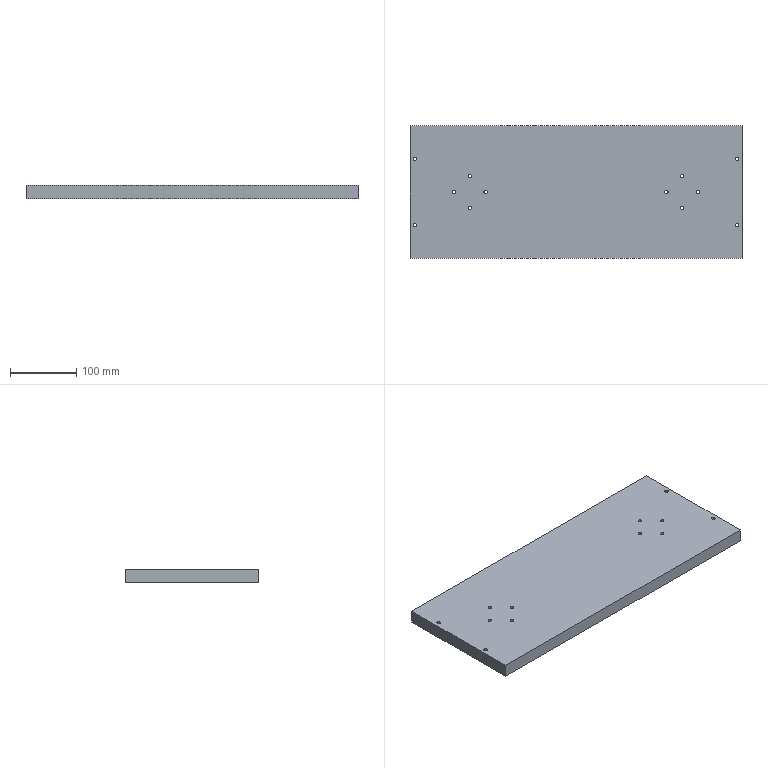Part | NX | features CBORE_HOLE 12, DATUM_CSYS 4, SKETCH 3, HOLE PACKAGE 2, EXTRUDE 1 | 1 solid | 42 faces | box 500 x 200 x 20 mm | volume 1988027 mm3 | cylinder 24 | plane 18 | commonest cylinder face diameters 5.2 x12 10 x12
STEP:
#1=CARTESIAN_POINT('',(-250.,100.,0.));
#2=VERTEX_POINT('',#1);
#3=CARTESIAN_POINT('',(-250.,-100.,0.));
#4=VERTEX_POINT('',#3);
#5=CARTESIAN_POINT('',(-250.,100.,0.));
#6=DIRECTION('',(0.,-1.,0.));
#7=VECTOR('',#6,1000.);
#8=LINE('',#5,#7);
#9=EDGE_CURVE('',#2,#4,#8,.T.);
#10=ORIENTED_EDGE('',*,*,#9,.T.);
#11=CARTESIAN_POINT('',(-250.,-100.,20.));
#12=VERTEX_POINT('',#11);
#13=CARTESIAN_POINT('',(-250.,-100.,20.));
#14=DIRECTION('',(0.,0.,-1.));
#15=VECTOR('',#14,1000.);
#16=LINE('',#13,#15);
#17=EDGE_CURVE('',#12,#4,#16,.T.);
#18=ORIENTED_EDGE('',*,*,#17,.F.);
#19=CARTESIAN_POINT('',(-250.,100.,20.));
#20=VERTEX_POINT('',#19);
#21=CARTESIAN_POINT('',(-250.,100.,20.));
#22=DIRECTION('',(0.,-1.,0.));
#23=VECTOR('',#22,1000.);
#24=LINE('',#21,#23);
#25=EDGE_CURVE('',#20,#12,#24,.T.);
#26=ORIENTED_EDGE('',*,*,#25,.F.);
#27=CARTESIAN_POINT('',(-250.,100.,20.));
#28=DIRECTION('',(0.,0.,-1.));
#29=VECTOR('',#28,1000.);
#30=LINE('',#27,#29);
#31=EDGE_CURVE('',#20,#2,#30,.T.);
#32=ORIENTED_EDGE('',*,*,#31,.T.);
#33=EDGE_LOOP('',(#10,#18,#26,#32));
#34=FACE_BOUND('',#33,.T.);
#35=CARTESIAN_POINT('',(-250.,100.,20.));
#36=DIRECTION('',(1.,0.,0.));
#37=DIRECTION('',(0.,1.,0.));
#38=AXIS2_PLACEMENT_3D('',#35,#36,#37);
#39=PLANE('',#38);
#40=ADVANCED_FACE('',(#34),#39,.F.);
#41=CARTESIAN_POINT('',(250.,-100.,0.));
#42=VERTEX_POINT('',#41);
#43=CARTESIAN_POINT('',(-250.,-100.,0.));
#44=DIRECTION('',(1.,0.,0.));
#45=VECTOR('',#44,1000.);
#46=LINE('',#43,#45);
#47=EDGE_CURVE('',#4,#42,#46,.T.);
#48=ORIENTED_EDGE('',*,*,#47,.T.);
#49=CARTESIAN_POINT('',(250.,-100.,20.));
#50=VERTEX_POINT('',#49);
#51=CARTESIAN_POINT('',(250.,-100.,20.));
#52=DIRECTION('',(0.,0.,-1.));
#53=VECTOR('',#52,1000.);
#54=LINE('',#51,#53);
#55=EDGE_CURVE('',#50,#42,#54,.T.);
#56=ORIENTED_EDGE('',*,*,#55,.F.);
#57=CARTESIAN_POINT('',(-250.,-100.,20.));
#58=DIRECTION('',(1.,0.,0.));
#59=VECTOR('',#58,1000.);
#60=LINE('',#57,#59);
#61=EDGE_CURVE('',#12,#50,#60,.T.);
#62=ORIENTED_EDGE('',*,*,#61,.F.);
#63=ORIENTED_EDGE('',*,*,#17,.T.);
#64=EDGE_LOOP('',(#48,#56,#62,#63));
#65=FACE_BOUND('',#64,.T.);
#66=CARTESIAN_POINT('',(-250.,-100.,20.));
#67=DIRECTION('',(0.,1.,0.));
#68=DIRECTION('',(0.,0.,1.));
#69=AXIS2_PLACEMENT_3D('',#66,#67,#68);
#70=PLANE('',#69);
#71=ADVANCED_FACE('',(#65),#70,.F.);
#72=CARTESIAN_POINT('',(250.,100.,0.));
#73=VERTEX_POINT('',#72);
#74=CARTESIAN_POINT('',(250.,-100.,0.));
#75=DIRECTION('',(0.,1.,0.));
#76=VECTOR('',#75,1000.);
#77=LINE('',#74,#76);
#78=EDGE_CURVE('',#42,#73,#77,.T.);
#79=ORIENTED_EDGE('',*,*,#78,.T.);
#80=CARTESIAN_POINT('',(250.,100.,20.));
#81=VERTEX_POINT('',#80);
#82=CARTESIAN_POINT('',(250.,100.,20.));
#83=DIRECTION('',(0.,0.,-1.));
#84=VECTOR('',#83,1000.);
#85=LINE('',#82,#84);
#86=EDGE_CURVE('',#81,#73,#85,.T.);
#87=ORIENTED_EDGE('',*,*,#86,.F.);
#88=CARTESIAN_POINT('',(250.,-100.,20.));
#89=DIRECTION('',(0.,1.,0.));
#90=VECTOR('',#89,1000.);
#91=LINE('',#88,#90);
#92=EDGE_CURVE('',#50,#81,#91,.T.);
#93=ORIENTED_EDGE('',*,*,#92,.F.);
#94=ORIENTED_EDGE('',*,*,#55,.T.);
#95=EDGE_LOOP('',(#79,#87,#93,#94));
#96=FACE_BOUND('',#95,.T.);
#97=CARTESIAN_POINT('',(250.,-100.,20.));
#98=DIRECTION('',(-1.,0.,0.));
#99=DIRECTION('',(0.,-1.,0.));
#100=AXIS2_PLACEMENT_3D('',#97,#98,#99);
#101=PLANE('',#100);
#102=ADVANCED_FACE('',(#96),#101,.F.);
#103=CARTESIAN_POINT('',(250.,100.,0.));
#104=DIRECTION('',(-1.,0.,0.));
#105=VECTOR('',#104,1000.);
#106=LINE('',#103,#105);
#107=EDGE_CURVE('',#73,#2,#106,.T.);
#108=ORIENTED_EDGE('',*,*,#107,.T.);
#109=ORIENTED_EDGE('',*,*,#31,.F.);
#110=CARTESIAN_POINT('',(250.,100.,20.));
#111=DIRECTION('',(-1.,0.,0.));
#112=VECTOR('',#111,1000.);
#113=LINE('',#110,#112);
#114=EDGE_CURVE('',#81,#20,#113,.T.);
#115=ORIENTED_EDGE('',*,*,#114,.F.);
#116=ORIENTED_EDGE('',*,*,#86,.T.);
#117=EDGE_LOOP('',(#108,#109,#115,#116));
#118=FACE_BOUND('',#117,.T.);
#119=CARTESIAN_POINT('',(250.,100.,20.));
#120=DIRECTION('',(0.,-1.,0.));
#121=DIRECTION('',(0.,0.,-1.));
#122=AXIS2_PLACEMENT_3D('',#119,#120,#121);
#123=PLANE('',#122);
#124=ADVANCED_FACE('',(#118),#123,.F.);
#125=CARTESIAN_POINT('',(-133.462,0.,20.));
#126=VERTEX_POINT('',#125);
#127=CARTESIAN_POINT('',(-136.062,0.,20.));
#128=DIRECTION('',(0.,0.,1.));
#129=DIRECTION('',(1.,0.,0.));
#130=AXIS2_PLACEMENT_3D('',#127,#128,#129);
#131=CIRCLE('',#130,2.6);
#132=EDGE_CURVE('',#126,#126,#131,.T.);
#133=ORIENTED_EDGE('',*,*,#132,.F.);
#134=EDGE_LOOP('',(#133));
#135=FACE_BOUND('',#134,.T.);
#136=CARTESIAN_POINT('',(-157.36,-23.75,20.));
#137=VERTEX_POINT('',#136);
#138=CARTESIAN_POINT('',(-159.96,-23.75,20.));
#139=DIRECTION('',(0.,0.,1.));
#140=DIRECTION('',(1.,0.,0.));
#141=AXIS2_PLACEMENT_3D('',#138,#139,#140);
#142=CIRCLE('',#141,2.6);
#143=EDGE_CURVE('',#137,#137,#142,.T.);
#144=ORIENTED_EDGE('',*,*,#143,.F.);
#145=EDGE_LOOP('',(#144));
#146=FACE_BOUND('',#145,.T.);
#147=CARTESIAN_POINT('',(-180.962,0.,20.));
#148=VERTEX_POINT('',#147);
#149=CARTESIAN_POINT('',(-183.562,0.,20.));
#150=DIRECTION('',(0.,0.,1.));
#151=DIRECTION('',(1.,0.,0.));
#152=AXIS2_PLACEMENT_3D('',#149,#150,#151);
#153=CIRCLE('',#152,2.6);
#154=EDGE_CURVE('',#148,#148,#153,.T.);
#155=ORIENTED_EDGE('',*,*,#154,.F.);
#156=EDGE_LOOP('',(#155));
#157=FACE_BOUND('',#156,.T.);
#158=CARTESIAN_POINT('',(-157.258,23.75,20.));
#159=VERTEX_POINT('',#158);
#160=CARTESIAN_POINT('',(-159.858,23.75,20.));
#161=DIRECTION('',(0.,0.,1.));
#162=DIRECTION('',(1.,0.,0.));
#163=AXIS2_PLACEMENT_3D('',#160,#161,#162);
#164=CIRCLE('',#163,2.6);
#165=EDGE_CURVE('',#159,#159,#164,.T.);
#166=ORIENTED_EDGE('',*,*,#165,.F.);
#167=EDGE_LOOP('',(#166));
#168=FACE_BOUND('',#167,.T.);
#169=CARTESIAN_POINT('',(138.662,0.,20.));
#170=VERTEX_POINT('',#169);
#171=CARTESIAN_POINT('',(136.062,0.,20.));
#172=DIRECTION('',(0.,0.,1.));
#173=DIRECTION('',(1.,0.,0.));
#174=AXIS2_PLACEMENT_3D('',#171,#172,#173);
#175=CIRCLE('',#174,2.6);
#176=EDGE_CURVE('',#170,#170,#175,.T.);
#177=ORIENTED_EDGE('',*,*,#176,.F.);
#178=EDGE_LOOP('',(#177));
#179=FACE_BOUND('',#178,.T.);
#180=CARTESIAN_POINT('',(162.56,-23.75,20.));
#181=VERTEX_POINT('',#180);
#182=CARTESIAN_POINT('',(159.96,-23.75,20.));
#183=DIRECTION('',(0.,0.,1.));
#184=DIRECTION('',(1.,0.,0.));
#185=AXIS2_PLACEMENT_3D('',#182,#183,#184);
#186=CIRCLE('',#185,2.6);
#187=EDGE_CURVE('',#181,#181,#186,.T.);
#188=ORIENTED_EDGE('',*,*,#187,.F.);
#189=EDGE_LOOP('',(#188));
#190=FACE_BOUND('',#189,.T.);
#191=CARTESIAN_POINT('',(186.162,0.,20.));
#192=VERTEX_POINT('',#191);
#193=CARTESIAN_POINT('',(183.562,0.,20.));
#194=DIRECTION('',(0.,0.,1.));
#195=DIRECTION('',(1.,0.,0.));
#196=AXIS2_PLACEMENT_3D('',#193,#194,#195);
#197=CIRCLE('',#196,2.6);
#198=EDGE_CURVE('',#192,#192,#197,.T.);
#199=ORIENTED_EDGE('',*,*,#198,.F.);
#200=EDGE_LOOP('',(#199));
#201=FACE_BOUND('',#200,.T.);
#202=CARTESIAN_POINT('',(162.458,23.75,20.));
#203=VERTEX_POINT('',#202);
#204=CARTESIAN_POINT('',(159.858,23.75,20.));
#205=DIRECTION('',(0.,0.,1.));
#206=DIRECTION('',(1.,0.,0.));
#207=AXIS2_PLACEMENT_3D('',#204,#205,#206);
#208=CIRCLE('',#207,2.6);
#209=EDGE_CURVE('',#203,#203,#208,.T.);
#210=ORIENTED_EDGE('',*,*,#209,.F.);
#211=EDGE_LOOP('',(#210));
#212=FACE_BOUND('',#211,.T.);
#213=CARTESIAN_POINT('',(-239.9,50.,20.));
#214=VERTEX_POINT('',#213);
#215=CARTESIAN_POINT('',(-242.5,50.,20.));
#216=DIRECTION('',(0.,0.,1.));
#217=DIRECTION('',(1.,0.,0.));
#218=AXIS2_PLACEMENT_3D('',#215,#216,#217);
#219=CIRCLE('',#218,2.6);
#220=EDGE_CURVE('',#214,#214,#219,.T.);
#221=ORIENTED_EDGE('',*,*,#220,.F.);
#222=EDGE_LOOP('',(#221));
#223=FACE_BOUND('',#222,.T.);
#224=CARTESIAN_POINT('',(-239.9,-50.,20.));
#225=VERTEX_POINT('',#224);
#226=CARTESIAN_POINT('',(-242.5,-50.,20.));
#227=DIRECTION('',(0.,0.,1.));
#228=DIRECTION('',(1.,0.,0.));
#229=AXIS2_PLACEMENT_3D('',#226,#227,#228);
#230=CIRCLE('',#229,2.6);
#231=EDGE_CURVE('',#225,#225,#230,.T.);
#232=ORIENTED_EDGE('',*,*,#231,.F.);
#233=EDGE_LOOP('',(#232));
#234=FACE_BOUND('',#233,.T.);
#235=CARTESIAN_POINT('',(245.1,50.,20.));
#236=VERTEX_POINT('',#235);
#237=CARTESIAN_POINT('',(242.5,50.,20.));
#238=DIRECTION('',(0.,0.,1.));
#239=DIRECTION('',(1.,0.,0.));
#240=AXIS2_PLACEMENT_3D('',#237,#238,#239);
#241=CIRCLE('',#240,2.6);
#242=EDGE_CURVE('',#236,#236,#241,.T.);
#243=ORIENTED_EDGE('',*,*,#242,.F.);
#244=EDGE_LOOP('',(#243));
#245=FACE_BOUND('',#244,.T.);
#246=CARTESIAN_POINT('',(245.1,-50.,20.));
#247=VERTEX_POINT('',#246);
#248=CARTESIAN_POINT('',(242.5,-50.,20.));
#249=DIRECTION('',(0.,0.,1.));
#250=DIRECTION('',(1.,0.,0.));
#251=AXIS2_PLACEMENT_3D('',#248,#249,#250);
#252=CIRCLE('',#251,2.6);
#253=EDGE_CURVE('',#247,#247,#252,.T.);
#254=ORIENTED_EDGE('',*,*,#253,.F.);
#255=EDGE_LOOP('',(#254));
#256=FACE_BOUND('',#255,.T.);
#257=ORIENTED_EDGE('',*,*,#25,.T.);
#258=ORIENTED_EDGE('',*,*,#61,.T.);
#259=ORIENTED_EDGE('',*,*,#92,.T.);
#260=ORIENTED_EDGE('',*,*,#114,.T.);
#261=EDGE_LOOP('',(#257,#258,#259,#260));
#262=FACE_BOUND('',#261,.T.);
#263=CARTESIAN_POINT('',(0.,0.,20.));
#264=DIRECTION('',(0.,0.,1.));
#265=DIRECTION('',(1.,0.,0.));
#266=AXIS2_PLACEMENT_3D('',#263,#264,#265);
#267=PLANE('',#266);
#268=ADVANCED_FACE('',(#135,#146,#157,#168,#179,#190,#201,#212,#223,#234,#245,#256,#262),#267,.T.);
#269=CARTESIAN_POINT('',(-131.062,0.,0.));
#270=VERTEX_POINT('',#269);
#271=CARTESIAN_POINT('',(-136.062,0.,0.));
#272=DIRECTION('',(0.,0.,1.));
#273=DIRECTION('',(1.,0.,0.));
#274=AXIS2_PLACEMENT_3D('',#271,#272,#273);
#275=CIRCLE('',#274,5.);
#276=EDGE_CURVE('',#270,#270,#275,.T.);
#277=ORIENTED_EDGE('',*,*,#276,.T.);
#278=EDGE_LOOP('',(#277));
#279=FACE_BOUND('',#278,.T.);
#280=CARTESIAN_POINT('',(-154.96,-23.75,0.));
#281=VERTEX_POINT('',#280);
#282=CARTESIAN_POINT('',(-159.96,-23.75,0.));
#283=DIRECTION('',(0.,0.,1.));
#284=DIRECTION('',(1.,0.,0.));
#285=AXIS2_PLACEMENT_3D('',#282,#283,#284);
#286=CIRCLE('',#285,5.);
#287=EDGE_CURVE('',#281,#281,#286,.T.);
#288=ORIENTED_EDGE('',*,*,#287,.T.);
#289=EDGE_LOOP('',(#288));
#290=FACE_BOUND('',#289,.T.);
#291=CARTESIAN_POINT('',(-178.562,0.,0.));
#292=VERTEX_POINT('',#291);
#293=CARTESIAN_POINT('',(-183.562,0.,0.));
#294=DIRECTION('',(0.,0.,1.));
#295=DIRECTION('',(1.,0.,0.));
#296=AXIS2_PLACEMENT_3D('',#293,#294,#295);
#297=CIRCLE('',#296,5.);
#298=EDGE_CURVE('',#292,#292,#297,.T.);
#299=ORIENTED_EDGE('',*,*,#298,.T.);
#300=EDGE_LOOP('',(#299));
#301=FACE_BOUND('',#300,.T.);
#302=CARTESIAN_POINT('',(-154.858,23.75,0.));
#303=VERTEX_POINT('',#302);
#304=CARTESIAN_POINT('',(-159.858,23.75,0.));
#305=DIRECTION('',(0.,0.,1.));
#306=DIRECTION('',(1.,0.,0.));
#307=AXIS2_PLACEMENT_3D('',#304,#305,#306);
#308=CIRCLE('',#307,5.);
#309=EDGE_CURVE('',#303,#303,#308,.T.);
#310=ORIENTED_EDGE('',*,*,#309,.T.);
#311=EDGE_LOOP('',(#310));
#312=FACE_BOUND('',#311,.T.);
#313=CARTESIAN_POINT('',(141.062,0.,0.));
#314=VERTEX_POINT('',#313);
#315=CARTESIAN_POINT('',(136.062,0.,0.));
#316=DIRECTION('',(0.,0.,1.));
#317=DIRECTION('',(1.,0.,0.));
#318=AXIS2_PLACEMENT_3D('',#315,#316,#317);
#319=CIRCLE('',#318,5.);
#320=EDGE_CURVE('',#314,#314,#319,.T.);
#321=ORIENTED_EDGE('',*,*,#320,.T.);
#322=EDGE_LOOP('',(#321));
#323=FACE_BOUND('',#322,.T.);
#324=CARTESIAN_POINT('',(164.96,-23.75,0.));
#325=VERTEX_POINT('',#324);
#326=CARTESIAN_POINT('',(159.96,-23.75,0.));
#327=DIRECTION('',(0.,0.,1.));
#328=DIRECTION('',(1.,0.,0.));
#329=AXIS2_PLACEMENT_3D('',#326,#327,#328);
#330=CIRCLE('',#329,5.);
#331=EDGE_CURVE('',#325,#325,#330,.T.);
#332=ORIENTED_EDGE('',*,*,#331,.T.);
#333=EDGE_LOOP('',(#332));
#334=FACE_BOUND('',#333,.T.);
#335=CARTESIAN_POINT('',(188.562,0.,0.));
#336=VERTEX_POINT('',#335);
#337=CARTESIAN_POINT('',(183.562,0.,0.));
#338=DIRECTION('',(0.,0.,1.));
#339=DIRECTION('',(1.,0.,0.));
#340=AXIS2_PLACEMENT_3D('',#337,#338,#339);
#341=CIRCLE('',#340,5.);
#342=EDGE_CURVE('',#336,#336,#341,.T.);
#343=ORIENTED_EDGE('',*,*,#342,.T.);
#344=EDGE_LOOP('',(#343));
#345=FACE_BOUND('',#344,.T.);
#346=CARTESIAN_POINT('',(164.858,23.75,0.));
#347=VERTEX_POINT('',#346);
#348=CARTESIAN_POINT('',(159.858,23.75,0.));
#349=DIRECTION('',(0.,0.,1.));
#350=DIRECTION('',(1.,0.,0.));
#351=AXIS2_PLACEMENT_3D('',#348,#349,#350);
#352=CIRCLE('',#351,5.);
#353=EDGE_CURVE('',#347,#347,#352,.T.);
#354=ORIENTED_EDGE('',*,*,#353,.T.);
#355=EDGE_LOOP('',(#354));
#356=FACE_BOUND('',#355,.T.);
#357=CARTESIAN_POINT('',(-237.5,50.,0.));
#358=VERTEX_POINT('',#357);
#359=CARTESIAN_POINT('',(-242.5,50.,0.));
#360=DIRECTION('',(0.,0.,1.));
#361=DIRECTION('',(1.,0.,0.));
#362=AXIS2_PLACEMENT_3D('',#359,#360,#361);
#363=CIRCLE('',#362,5.);
#364=EDGE_CURVE('',#358,#358,#363,.T.);
#365=ORIENTED_EDGE('',*,*,#364,.T.);
#366=EDGE_LOOP('',(#365));
#367=FACE_BOUND('',#366,.T.);
#368=CARTESIAN_POINT('',(-237.5,-50.,0.));
#369=VERTEX_POINT('',#368);
#370=CARTESIAN_POINT('',(-242.5,-50.,0.));
#371=DIRECTION('',(0.,0.,1.));
#372=DIRECTION('',(1.,0.,0.));
#373=AXIS2_PLACEMENT_3D('',#370,#371,#372);
#374=CIRCLE('',#373,5.);
#375=EDGE_CURVE('',#369,#369,#374,.T.);
#376=ORIENTED_EDGE('',*,*,#375,.T.);
#377=EDGE_LOOP('',(#376));
#378=FACE_BOUND('',#377,.T.);
#379=CARTESIAN_POINT('',(247.5,50.,0.));
#380=VERTEX_POINT('',#379);
#381=CARTESIAN_POINT('',(242.5,50.,0.));
#382=DIRECTION('',(0.,0.,1.));
#383=DIRECTION('',(1.,0.,0.));
#384=AXIS2_PLACEMENT_3D('',#381,#382,#383);
#385=CIRCLE('',#384,5.);
#386=EDGE_CURVE('',#380,#380,#385,.T.);
#387=ORIENTED_EDGE('',*,*,#386,.T.);
#388=EDGE_LOOP('',(#387));
#389=FACE_BOUND('',#388,.T.);
#390=CARTESIAN_POINT('',(247.5,-50.,0.));
#391=VERTEX_POINT('',#390);
#392=CARTESIAN_POINT('',(242.5,-50.,0.));
#393=DIRECTION('',(0.,0.,1.));
#394=DIRECTION('',(1.,0.,0.));
#395=AXIS2_PLACEMENT_3D('',#392,#393,#394);
#396=CIRCLE('',#395,5.);
#397=EDGE_CURVE('',#391,#391,#396,.T.);
#398=ORIENTED_EDGE('',*,*,#397,.T.);
#399=EDGE_LOOP('',(#398));
#400=FACE_BOUND('',#399,.T.);
#401=ORIENTED_EDGE('',*,*,#9,.F.);
#402=ORIENTED_EDGE('',*,*,#107,.F.);
#403=ORIENTED_EDGE('',*,*,#78,.F.);
#404=ORIENTED_EDGE('',*,*,#47,.F.);
#405=EDGE_LOOP('',(#401,#402,#403,#404));
#406=FACE_BOUND('',#405,.T.);
#407=CARTESIAN_POINT('',(0.,0.,0.));
#408=DIRECTION('',(0.,0.,1.));
#409=DIRECTION('',(1.,0.,0.));
#410=AXIS2_PLACEMENT_3D('',#407,#408,#409);
#411=PLANE('',#410);
#412=ADVANCED_FACE('',(#279,#290,#301,#312,#323,#334,#345,#356,#367,#378,#389,#400,#406),#411,.F.);
#413=ORIENTED_EDGE('',*,*,#253,.T.);
#414=EDGE_LOOP('',(#413));
#415=FACE_BOUND('',#414,.T.);
#416=CARTESIAN_POINT('',(245.1,-50.,10.));
#417=VERTEX_POINT('',#416);
#418=CARTESIAN_POINT('',(242.5,-50.,10.));
#419=DIRECTION('',(0.,0.,1.));
#420=DIRECTION('',(1.,0.,0.));
#421=AXIS2_PLACEMENT_3D('',#418,#419,#420);
#422=CIRCLE('',#421,2.6);
#423=EDGE_CURVE('',#417,#417,#422,.F.);
#424=ORIENTED_EDGE('',*,*,#423,.T.);
#425=EDGE_LOOP('',(#424));
#426=FACE_BOUND('',#425,.T.);
#427=CARTESIAN_POINT('',(242.5,-50.,50.));
#428=DIRECTION('',(0.,0.,1.));
#429=DIRECTION('',(1.,0.,0.));
#430=AXIS2_PLACEMENT_3D('',#427,#428,#429);
#431=CYLINDRICAL_SURFACE('',#430,2.6);
#432=ADVANCED_FACE('',(#415,#426),#431,.F.);
#433=ORIENTED_EDGE('',*,*,#423,.F.);
#434=EDGE_LOOP('',(#433));
#435=FACE_BOUND('',#434,.T.);
#436=CARTESIAN_POINT('',(247.5,-50.,10.));
#437=VERTEX_POINT('',#436);
#438=CARTESIAN_POINT('',(242.5,-50.,10.));
#439=DIRECTION('',(0.,0.,1.));
#440=DIRECTION('',(1.,0.,0.));
#441=AXIS2_PLACEMENT_3D('',#438,#439,#440);
#442=CIRCLE('',#441,5.);
#443=EDGE_CURVE('',#437,#437,#442,.F.);
#444=ORIENTED_EDGE('',*,*,#443,.T.);
#445=EDGE_LOOP('',(#444));
#446=FACE_BOUND('',#445,.T.);
#447=CARTESIAN_POINT('',(242.5,-50.,10.));
#448=DIRECTION('',(0.,0.,1.));
#449=DIRECTION('',(1.,0.,0.));
#450=AXIS2_PLACEMENT_3D('',#447,#448,#449);
#451=PLANE('',#450);
#452=ADVANCED_FACE('',(#435,#446),#451,.F.);
#453=ORIENTED_EDGE('',*,*,#443,.F.);
#454=EDGE_LOOP('',(#453));
#455=FACE_BOUND('',#454,.T.);
#456=ORIENTED_EDGE('',*,*,#397,.F.);
#457=EDGE_LOOP('',(#456));
#458=FACE_BOUND('',#457,.T.);
#459=CARTESIAN_POINT('',(242.5,-50.,0.));
#460=DIRECTION('',(0.,0.,1.));
#461=DIRECTION('',(1.,0.,0.));
#462=AXIS2_PLACEMENT_3D('',#459,#460,#461);
#463=CYLINDRICAL_SURFACE('',#462,5.);
#464=ADVANCED_FACE('',(#455,#458),#463,.F.);
#465=ORIENTED_EDGE('',*,*,#242,.T.);
#466=EDGE_LOOP('',(#465));
#467=FACE_BOUND('',#466,.T.);
#468=CARTESIAN_POINT('',(245.1,50.,10.));
#469=VERTEX_POINT('',#468);
#470=CARTESIAN_POINT('',(242.5,50.,10.));
#471=DIRECTION('',(0.,0.,1.));
#472=DIRECTION('',(1.,0.,0.));
#473=AXIS2_PLACEMENT_3D('',#470,#471,#472);
#474=CIRCLE('',#473,2.6);
#475=EDGE_CURVE('',#469,#469,#474,.F.);
#476=ORIENTED_EDGE('',*,*,#475,.T.);
#477=EDGE_LOOP('',(#476));
#478=FACE_BOUND('',#477,.T.);
#479=CARTESIAN_POINT('',(242.5,50.,50.));
#480=DIRECTION('',(0.,0.,1.));
#481=DIRECTION('',(1.,0.,0.));
#482=AXIS2_PLACEMENT_3D('',#479,#480,#481);
#483=CYLINDRICAL_SURFACE('',#482,2.6);
#484=ADVANCED_FACE('',(#467,#478),#483,.F.);
#485=ORIENTED_EDGE('',*,*,#475,.F.);
#486=EDGE_LOOP('',(#485));
#487=FACE_BOUND('',#486,.T.);
#488=CARTESIAN_POINT('',(247.5,50.,10.));
#489=VERTEX_POINT('',#488);
#490=CARTESIAN_POINT('',(242.5,50.,10.));
#491=DIRECTION('',(0.,0.,1.));
#492=DIRECTION('',(1.,0.,0.));
#493=AXIS2_PLACEMENT_3D('',#490,#491,#492);
#494=CIRCLE('',#493,5.);
#495=EDGE_CURVE('',#489,#489,#494,.F.);
#496=ORIENTED_EDGE('',*,*,#495,.T.);
#497=EDGE_LOOP('',(#496));
#498=FACE_BOUND('',#497,.T.);
#499=CARTESIAN_POINT('',(242.5,50.,10.));
#500=DIRECTION('',(0.,0.,1.));
#501=DIRECTION('',(1.,0.,0.));
#502=AXIS2_PLACEMENT_3D('',#499,#500,#501);
#503=PLANE('',#502);
#504=ADVANCED_FACE('',(#487,#498),#503,.F.);
#505=ORIENTED_EDGE('',*,*,#495,.F.);
#506=EDGE_LOOP('',(#505));
#507=FACE_BOUND('',#506,.T.);
#508=ORIENTED_EDGE('',*,*,#386,.F.);
#509=EDGE_LOOP('',(#508));
#510=FACE_BOUND('',#509,.T.);
#511=CARTESIAN_POINT('',(242.5,50.,0.));
#512=DIRECTION('',(0.,0.,1.));
#513=DIRECTION('',(1.,0.,0.));
#514=AXIS2_PLACEMENT_3D('',#511,#512,#513);
#515=CYLINDRICAL_SURFACE('',#514,5.);
#516=ADVANCED_FACE('',(#507,#510),#515,.F.);
#517=ORIENTED_EDGE('',*,*,#231,.T.);
#518=EDGE_LOOP('',(#517));
#519=FACE_BOUND('',#518,.T.);
#520=CARTESIAN_POINT('',(-239.9,-50.,10.));
#521=VERTEX_POINT('',#520);
#522=CARTESIAN_POINT('',(-242.5,-50.,10.));
#523=DIRECTION('',(0.,0.,1.));
#524=DIRECTION('',(1.,0.,0.));
#525=AXIS2_PLACEMENT_3D('',#522,#523,#524);
#526=CIRCLE('',#525,2.6);
#527=EDGE_CURVE('',#521,#521,#526,.F.);
#528=ORIENTED_EDGE('',*,*,#527,.T.);
#529=EDGE_LOOP('',(#528));
#530=FACE_BOUND('',#529,.T.);
#531=CARTESIAN_POINT('',(-242.5,-50.,50.));
#532=DIRECTION('',(0.,0.,1.));
#533=DIRECTION('',(1.,0.,0.));
#534=AXIS2_PLACEMENT_3D('',#531,#532,#533);
#535=CYLINDRICAL_SURFACE('',#534,2.6);
#536=ADVANCED_FACE('',(#519,#530),#535,.F.);
#537=ORIENTED_EDGE('',*,*,#527,.F.);
#538=EDGE_LOOP('',(#537));
#539=FACE_BOUND('',#538,.T.);
#540=CARTESIAN_POINT('',(-237.5,-50.,10.));
#541=VERTEX_POINT('',#540);
#542=CARTESIAN_POINT('',(-242.5,-50.,10.));
#543=DIRECTION('',(0.,0.,1.));
#544=DIRECTION('',(1.,0.,0.));
#545=AXIS2_PLACEMENT_3D('',#542,#543,#544);
#546=CIRCLE('',#545,5.);
#547=EDGE_CURVE('',#541,#541,#546,.F.);
#548=ORIENTED_EDGE('',*,*,#547,.T.);
#549=EDGE_LOOP('',(#548));
#550=FACE_BOUND('',#549,.T.);
#551=CARTESIAN_POINT('',(-242.5,-50.,10.));
#552=DIRECTION('',(0.,0.,1.));
#553=DIRECTION('',(1.,0.,0.));
#554=AXIS2_PLACEMENT_3D('',#551,#552,#553);
#555=PLANE('',#554);
#556=ADVANCED_FACE('',(#539,#550),#555,.F.);
#557=ORIENTED_EDGE('',*,*,#547,.F.);
#558=EDGE_LOOP('',(#557));
#559=FACE_BOUND('',#558,.T.);
#560=ORIENTED_EDGE('',*,*,#375,.F.);
#561=EDGE_LOOP('',(#560));
#562=FACE_BOUND('',#561,.T.);
#563=CARTESIAN_POINT('',(-242.5,-50.,0.));
#564=DIRECTION('',(0.,0.,1.));
#565=DIRECTION('',(1.,0.,0.));
#566=AXIS2_PLACEMENT_3D('',#563,#564,#565);
#567=CYLINDRICAL_SURFACE('',#566,5.);
#568=ADVANCED_FACE('',(#559,#562),#567,.F.);
#569=ORIENTED_EDGE('',*,*,#220,.T.);
#570=EDGE_LOOP('',(#569));
#571=FACE_BOUND('',#570,.T.);
#572=CARTESIAN_POINT('',(-239.9,50.,10.));
#573=VERTEX_POINT('',#572);
#574=CARTESIAN_POINT('',(-242.5,50.,10.));
#575=DIRECTION('',(0.,0.,1.));
#576=DIRECTION('',(1.,0.,0.));
#577=AXIS2_PLACEMENT_3D('',#574,#575,#576);
#578=CIRCLE('',#577,2.6);
#579=EDGE_CURVE('',#573,#573,#578,.F.);
#580=ORIENTED_EDGE('',*,*,#579,.T.);
#581=EDGE_LOOP('',(#580));
#582=FACE_BOUND('',#581,.T.);
#583=CARTESIAN_POINT('',(-242.5,50.,50.));
#584=DIRECTION('',(0.,0.,1.));
#585=DIRECTION('',(1.,0.,0.));
#586=AXIS2_PLACEMENT_3D('',#583,#584,#585);
#587=CYLINDRICAL_SURFACE('',#586,2.6);
#588=ADVANCED_FACE('',(#571,#582),#587,.F.);
#589=ORIENTED_EDGE('',*,*,#579,.F.);
#590=EDGE_LOOP('',(#589));
#591=FACE_BOUND('',#590,.T.);
#592=CARTESIAN_POINT('',(-237.5,50.,10.));
#593=VERTEX_POINT('',#592);
#594=CARTESIAN_POINT('',(-242.5,50.,10.));
#595=DIRECTION('',(0.,0.,1.));
#596=DIRECTION('',(1.,0.,0.));
#597=AXIS2_PLACEMENT_3D('',#594,#595,#596);
#598=CIRCLE('',#597,5.);
#599=EDGE_CURVE('',#593,#593,#598,.F.);
#600=ORIENTED_EDGE('',*,*,#599,.T.);
#601=EDGE_LOOP('',(#600));
#602=FACE_BOUND('',#601,.T.);
#603=CARTESIAN_POINT('',(-242.5,50.,10.));
#604=DIRECTION('',(0.,0.,1.));
#605=DIRECTION('',(1.,0.,0.));
#606=AXIS2_PLACEMENT_3D('',#603,#604,#605);
#607=PLANE('',#606);
#608=ADVANCED_FACE('',(#591,#602),#607,.F.);
#609=ORIENTED_EDGE('',*,*,#599,.F.);
#610=EDGE_LOOP('',(#609));
#611=FACE_BOUND('',#610,.T.);
#612=ORIENTED_EDGE('',*,*,#364,.F.);
#613=EDGE_LOOP('',(#612));
#614=FACE_BOUND('',#613,.T.);
#615=CARTESIAN_POINT('',(-242.5,50.,0.));
#616=DIRECTION('',(0.,0.,1.));
#617=DIRECTION('',(1.,0.,0.));
#618=AXIS2_PLACEMENT_3D('',#615,#616,#617);
#619=CYLINDRICAL_SURFACE('',#618,5.);
#620=ADVANCED_FACE('',(#611,#614),#619,.F.);
#621=ORIENTED_EDGE('',*,*,#209,.T.);
#622=EDGE_LOOP('',(#621));
#623=FACE_BOUND('',#622,.T.);
#624=CARTESIAN_POINT('',(162.458,23.75,10.));
#625=VERTEX_POINT('',#624);
#626=CARTESIAN_POINT('',(159.858,23.75,10.));
#627=DIRECTION('',(0.,0.,1.));
#628=DIRECTION('',(1.,0.,0.));
#629=AXIS2_PLACEMENT_3D('',#626,#627,#628);
#630=CIRCLE('',#629,2.6);
#631=EDGE_CURVE('',#625,#625,#630,.F.);
#632=ORIENTED_EDGE('',*,*,#631,.T.);
#633=EDGE_LOOP('',(#632));
#634=FACE_BOUND('',#633,.T.);
#635=CARTESIAN_POINT('',(159.858,23.75,50.));
#636=DIRECTION('',(0.,0.,1.));
#637=DIRECTION('',(1.,0.,0.));
#638=AXIS2_PLACEMENT_3D('',#635,#636,#637);
#639=CYLINDRICAL_SURFACE('',#638,2.6);
#640=ADVANCED_FACE('',(#623,#634),#639,.F.);
#641=ORIENTED_EDGE('',*,*,#631,.F.);
#642=EDGE_LOOP('',(#641));
#643=FACE_BOUND('',#642,.T.);
#644=CARTESIAN_POINT('',(164.858,23.75,10.));
#645=VERTEX_POINT('',#644);
#646=CARTESIAN_POINT('',(159.858,23.75,10.));
#647=DIRECTION('',(0.,0.,1.));
#648=DIRECTION('',(1.,0.,0.));
#649=AXIS2_PLACEMENT_3D('',#646,#647,#648);
#650=CIRCLE('',#649,5.);
#651=EDGE_CURVE('',#645,#645,#650,.F.);
#652=ORIENTED_EDGE('',*,*,#651,.T.);
#653=EDGE_LOOP('',(#652));
#654=FACE_BOUND('',#653,.T.);
#655=CARTESIAN_POINT('',(159.858,23.75,10.));
#656=DIRECTION('',(0.,0.,1.));
#657=DIRECTION('',(1.,0.,0.));
#658=AXIS2_PLACEMENT_3D('',#655,#656,#657);
#659=PLANE('',#658);
#660=ADVANCED_FACE('',(#643,#654),#659,.F.);
#661=ORIENTED_EDGE('',*,*,#651,.F.);
#662=EDGE_LOOP('',(#661));
#663=FACE_BOUND('',#662,.T.);
#664=ORIENTED_EDGE('',*,*,#353,.F.);
#665=EDGE_LOOP('',(#664));
#666=FACE_BOUND('',#665,.T.);
#667=CARTESIAN_POINT('',(159.858,23.75,0.));
#668=DIRECTION('',(0.,0.,1.));
#669=DIRECTION('',(1.,0.,0.));
#670=AXIS2_PLACEMENT_3D('',#667,#668,#669);
#671=CYLINDRICAL_SURFACE('',#670,5.);
#672=ADVANCED_FACE('',(#663,#666),#671,.F.);
#673=ORIENTED_EDGE('',*,*,#198,.T.);
#674=EDGE_LOOP('',(#673));
#675=FACE_BOUND('',#674,.T.);
#676=CARTESIAN_POINT('',(186.162,0.,10.));
#677=VERTEX_POINT('',#676);
#678=CARTESIAN_POINT('',(183.562,0.,10.));
#679=DIRECTION('',(0.,0.,1.));
#680=DIRECTION('',(1.,0.,0.));
#681=AXIS2_PLACEMENT_3D('',#678,#679,#680);
#682=CIRCLE('',#681,2.6);
#683=EDGE_CURVE('',#677,#677,#682,.F.);
#684=ORIENTED_EDGE('',*,*,#683,.T.);
#685=EDGE_LOOP('',(#684));
#686=FACE_BOUND('',#685,.T.);
#687=CARTESIAN_POINT('',(183.562,0.,50.));
#688=DIRECTION('',(0.,0.,1.));
#689=DIRECTION('',(1.,0.,0.));
#690=AXIS2_PLACEMENT_3D('',#687,#688,#689);
#691=CYLINDRICAL_SURFACE('',#690,2.6);
#692=ADVANCED_FACE('',(#675,#686),#691,.F.);
#693=ORIENTED_EDGE('',*,*,#683,.F.);
#694=EDGE_LOOP('',(#693));
#695=FACE_BOUND('',#694,.T.);
#696=CARTESIAN_POINT('',(188.562,0.,10.));
#697=VERTEX_POINT('',#696);
#698=CARTESIAN_POINT('',(183.562,0.,10.));
#699=DIRECTION('',(0.,0.,1.));
#700=DIRECTION('',(1.,0.,0.));
#701=AXIS2_PLACEMENT_3D('',#698,#699,#700);
#702=CIRCLE('',#701,5.);
#703=EDGE_CURVE('',#697,#697,#702,.F.);
#704=ORIENTED_EDGE('',*,*,#703,.T.);
#705=EDGE_LOOP('',(#704));
#706=FACE_BOUND('',#705,.T.);
#707=CARTESIAN_POINT('',(183.562,0.,10.));
#708=DIRECTION('',(0.,0.,1.));
#709=DIRECTION('',(1.,0.,0.));
#710=AXIS2_PLACEMENT_3D('',#707,#708,#709);
#711=PLANE('',#710);
#712=ADVANCED_FACE('',(#695,#706),#711,.F.);
#713=ORIENTED_EDGE('',*,*,#703,.F.);
#714=EDGE_LOOP('',(#713));
#715=FACE_BOUND('',#714,.T.);
#716=ORIENTED_EDGE('',*,*,#342,.F.);
#717=EDGE_LOOP('',(#716));
#718=FACE_BOUND('',#717,.T.);
#719=CARTESIAN_POINT('',(183.562,0.,0.));
#720=DIRECTION('',(0.,0.,1.));
#721=DIRECTION('',(1.,0.,0.));
#722=AXIS2_PLACEMENT_3D('',#719,#720,#721);
#723=CYLINDRICAL_SURFACE('',#722,5.);
#724=ADVANCED_FACE('',(#715,#718),#723,.F.);
#725=ORIENTED_EDGE('',*,*,#187,.T.);
#726=EDGE_LOOP('',(#725));
#727=FACE_BOUND('',#726,.T.);
#728=CARTESIAN_POINT('',(162.56,-23.75,10.));
#729=VERTEX_POINT('',#728);
#730=CARTESIAN_POINT('',(159.96,-23.75,10.));
#731=DIRECTION('',(0.,0.,1.));
#732=DIRECTION('',(1.,0.,0.));
#733=AXIS2_PLACEMENT_3D('',#730,#731,#732);
#734=CIRCLE('',#733,2.6);
#735=EDGE_CURVE('',#729,#729,#734,.F.);
#736=ORIENTED_EDGE('',*,*,#735,.T.);
#737=EDGE_LOOP('',(#736));
#738=FACE_BOUND('',#737,.T.);
#739=CARTESIAN_POINT('',(159.96,-23.75,50.));
#740=DIRECTION('',(0.,0.,1.));
#741=DIRECTION('',(1.,0.,0.));
#742=AXIS2_PLACEMENT_3D('',#739,#740,#741);
#743=CYLINDRICAL_SURFACE('',#742,2.6);
#744=ADVANCED_FACE('',(#727,#738),#743,.F.);
#745=ORIENTED_EDGE('',*,*,#735,.F.);
#746=EDGE_LOOP('',(#745));
#747=FACE_BOUND('',#746,.T.);
#748=CARTESIAN_POINT('',(164.96,-23.75,10.));
#749=VERTEX_POINT('',#748);
#750=CARTESIAN_POINT('',(159.96,-23.75,10.));
#751=DIRECTION('',(0.,0.,1.));
#752=DIRECTION('',(1.,0.,0.));
#753=AXIS2_PLACEMENT_3D('',#750,#751,#752);
#754=CIRCLE('',#753,5.);
#755=EDGE_CURVE('',#749,#749,#754,.F.);
#756=ORIENTED_EDGE('',*,*,#755,.T.);
#757=EDGE_LOOP('',(#756));
#758=FACE_BOUND('',#757,.T.);
#759=CARTESIAN_POINT('',(159.96,-23.75,10.));
#760=DIRECTION('',(0.,0.,1.));
#761=DIRECTION('',(1.,0.,0.));
#762=AXIS2_PLACEMENT_3D('',#759,#760,#761);
#763=PLANE('',#762);
#764=ADVANCED_FACE('',(#747,#758),#763,.F.);
#765=ORIENTED_EDGE('',*,*,#755,.F.);
#766=EDGE_LOOP('',(#765));
#767=FACE_BOUND('',#766,.T.);
#768=ORIENTED_EDGE('',*,*,#331,.F.);
#769=EDGE_LOOP('',(#768));
#770=FACE_BOUND('',#769,.T.);
#771=CARTESIAN_POINT('',(159.96,-23.75,0.));
#772=DIRECTION('',(0.,0.,1.));
#773=DIRECTION('',(1.,0.,0.));
#774=AXIS2_PLACEMENT_3D('',#771,#772,#773);
#775=CYLINDRICAL_SURFACE('',#774,5.);
#776=ADVANCED_FACE('',(#767,#770),#775,.F.);
#777=ORIENTED_EDGE('',*,*,#176,.T.);
#778=EDGE_LOOP('',(#777));
#779=FACE_BOUND('',#778,.T.);
#780=CARTESIAN_POINT('',(138.662,0.,10.));
#781=VERTEX_POINT('',#780);
#782=CARTESIAN_POINT('',(136.062,0.,10.));
#783=DIRECTION('',(0.,0.,1.));
#784=DIRECTION('',(1.,0.,0.));
#785=AXIS2_PLACEMENT_3D('',#782,#783,#784);
#786=CIRCLE('',#785,2.6);
#787=EDGE_CURVE('',#781,#781,#786,.F.);
#788=ORIENTED_EDGE('',*,*,#787,.T.);
#789=EDGE_LOOP('',(#788));
#790=FACE_BOUND('',#789,.T.);
#791=CARTESIAN_POINT('',(136.062,0.,50.));
#792=DIRECTION('',(0.,0.,1.));
#793=DIRECTION('',(1.,0.,0.));
#794=AXIS2_PLACEMENT_3D('',#791,#792,#793);
#795=CYLINDRICAL_SURFACE('',#794,2.6);
#796=ADVANCED_FACE('',(#779,#790),#795,.F.);
#797=ORIENTED_EDGE('',*,*,#787,.F.);
#798=EDGE_LOOP('',(#797));
#799=FACE_BOUND('',#798,.T.);
#800=CARTESIAN_POINT('',(141.062,0.,10.));
#801=VERTEX_POINT('',#800);
#802=CARTESIAN_POINT('',(136.062,0.,10.));
#803=DIRECTION('',(0.,0.,1.));
#804=DIRECTION('',(1.,0.,0.));
#805=AXIS2_PLACEMENT_3D('',#802,#803,#804);
#806=CIRCLE('',#805,5.);
#807=EDGE_CURVE('',#801,#801,#806,.F.);
#808=ORIENTED_EDGE('',*,*,#807,.T.);
#809=EDGE_LOOP('',(#808));
#810=FACE_BOUND('',#809,.T.);
#811=CARTESIAN_POINT('',(136.062,0.,10.));
#812=DIRECTION('',(0.,0.,1.));
#813=DIRECTION('',(1.,0.,0.));
#814=AXIS2_PLACEMENT_3D('',#811,#812,#813);
#815=PLANE('',#814);
#816=ADVANCED_FACE('',(#799,#810),#815,.F.);
#817=ORIENTED_EDGE('',*,*,#807,.F.);
#818=EDGE_LOOP('',(#817));
#819=FACE_BOUND('',#818,.T.);
#820=ORIENTED_EDGE('',*,*,#320,.F.);
#821=EDGE_LOOP('',(#820));
#822=FACE_BOUND('',#821,.T.);
#823=CARTESIAN_POINT('',(136.062,0.,0.));
#824=DIRECTION('',(0.,0.,1.));
#825=DIRECTION('',(1.,0.,0.));
#826=AXIS2_PLACEMENT_3D('',#823,#824,#825);
#827=CYLINDRICAL_SURFACE('',#826,5.);
#828=ADVANCED_FACE('',(#819,#822),#827,.F.);
#829=ORIENTED_EDGE('',*,*,#165,.T.);
#830=EDGE_LOOP('',(#829));
#831=FACE_BOUND('',#830,.T.);
#832=CARTESIAN_POINT('',(-157.258,23.75,10.));
#833=VERTEX_POINT('',#832);
#834=CARTESIAN_POINT('',(-159.858,23.75,10.));
#835=DIRECTION('',(0.,0.,1.));
#836=DIRECTION('',(1.,0.,0.));
#837=AXIS2_PLACEMENT_3D('',#834,#835,#836);
#838=CIRCLE('',#837,2.6);
#839=EDGE_CURVE('',#833,#833,#838,.F.);
#840=ORIENTED_EDGE('',*,*,#839,.T.);
#841=EDGE_LOOP('',(#840));
#842=FACE_BOUND('',#841,.T.);
#843=CARTESIAN_POINT('',(-159.858,23.75,50.));
#844=DIRECTION('',(0.,0.,1.));
#845=DIRECTION('',(1.,0.,0.));
#846=AXIS2_PLACEMENT_3D('',#843,#844,#845);
#847=CYLINDRICAL_SURFACE('',#846,2.6);
#848=ADVANCED_FACE('',(#831,#842),#847,.F.);
#849=ORIENTED_EDGE('',*,*,#839,.F.);
#850=EDGE_LOOP('',(#849));
#851=FACE_BOUND('',#850,.T.);
#852=CARTESIAN_POINT('',(-154.858,23.75,10.));
#853=VERTEX_POINT('',#852);
#854=CARTESIAN_POINT('',(-159.858,23.75,10.));
#855=DIRECTION('',(0.,0.,1.));
#856=DIRECTION('',(1.,0.,0.));
#857=AXIS2_PLACEMENT_3D('',#854,#855,#856);
#858=CIRCLE('',#857,5.);
#859=EDGE_CURVE('',#853,#853,#858,.F.);
#860=ORIENTED_EDGE('',*,*,#859,.T.);
#861=EDGE_LOOP('',(#860));
#862=FACE_BOUND('',#861,.T.);
#863=CARTESIAN_POINT('',(-159.858,23.75,10.));
#864=DIRECTION('',(0.,0.,1.));
#865=DIRECTION('',(1.,0.,0.));
#866=AXIS2_PLACEMENT_3D('',#863,#864,#865);
#867=PLANE('',#866);
#868=ADVANCED_FACE('',(#851,#862),#867,.F.);
#869=ORIENTED_EDGE('',*,*,#859,.F.);
#870=EDGE_LOOP('',(#869));
#871=FACE_BOUND('',#870,.T.);
#872=ORIENTED_EDGE('',*,*,#309,.F.);
#873=EDGE_LOOP('',(#872));
#874=FACE_BOUND('',#873,.T.);
#875=CARTESIAN_POINT('',(-159.858,23.75,0.));
#876=DIRECTION('',(0.,0.,1.));
#877=DIRECTION('',(1.,0.,0.));
#878=AXIS2_PLACEMENT_3D('',#875,#876,#877);
#879=CYLINDRICAL_SURFACE('',#878,5.);
#880=ADVANCED_FACE('',(#871,#874),#879,.F.);
#881=ORIENTED_EDGE('',*,*,#154,.T.);
#882=EDGE_LOOP('',(#881));
#883=FACE_BOUND('',#882,.T.);
#884=CARTESIAN_POINT('',(-180.962,0.,10.));
#885=VERTEX_POINT('',#884);
#886=CARTESIAN_POINT('',(-183.562,0.,10.));
#887=DIRECTION('',(0.,0.,1.));
#888=DIRECTION('',(1.,0.,0.));
#889=AXIS2_PLACEMENT_3D('',#886,#887,#888);
#890=CIRCLE('',#889,2.6);
#891=EDGE_CURVE('',#885,#885,#890,.F.);
#892=ORIENTED_EDGE('',*,*,#891,.T.);
#893=EDGE_LOOP('',(#892));
#894=FACE_BOUND('',#893,.T.);
#895=CARTESIAN_POINT('',(-183.562,0.,50.));
#896=DIRECTION('',(0.,0.,1.));
#897=DIRECTION('',(1.,0.,0.));
#898=AXIS2_PLACEMENT_3D('',#895,#896,#897);
#899=CYLINDRICAL_SURFACE('',#898,2.6);
#900=ADVANCED_FACE('',(#883,#894),#899,.F.);
#901=ORIENTED_EDGE('',*,*,#891,.F.);
#902=EDGE_LOOP('',(#901));
#903=FACE_BOUND('',#902,.T.);
#904=CARTESIAN_POINT('',(-178.562,0.,10.));
#905=VERTEX_POINT('',#904);
#906=CARTESIAN_POINT('',(-183.562,0.,10.));
#907=DIRECTION('',(0.,0.,1.));
#908=DIRECTION('',(1.,0.,0.));
#909=AXIS2_PLACEMENT_3D('',#906,#907,#908);
#910=CIRCLE('',#909,5.);
#911=EDGE_CURVE('',#905,#905,#910,.F.);
#912=ORIENTED_EDGE('',*,*,#911,.T.);
#913=EDGE_LOOP('',(#912));
#914=FACE_BOUND('',#913,.T.);
#915=CARTESIAN_POINT('',(-183.562,0.,10.));
#916=DIRECTION('',(0.,0.,1.));
#917=DIRECTION('',(1.,0.,0.));
#918=AXIS2_PLACEMENT_3D('',#915,#916,#917);
#919=PLANE('',#918);
#920=ADVANCED_FACE('',(#903,#914),#919,.F.);
#921=ORIENTED_EDGE('',*,*,#911,.F.);
#922=EDGE_LOOP('',(#921));
#923=FACE_BOUND('',#922,.T.);
#924=ORIENTED_EDGE('',*,*,#298,.F.);
#925=EDGE_LOOP('',(#924));
#926=FACE_BOUND('',#925,.T.);
#927=CARTESIAN_POINT('',(-183.562,0.,0.));
#928=DIRECTION('',(0.,0.,1.));
#929=DIRECTION('',(1.,0.,0.));
#930=AXIS2_PLACEMENT_3D('',#927,#928,#929);
#931=CYLINDRICAL_SURFACE('',#930,5.);
#932=ADVANCED_FACE('',(#923,#926),#931,.F.);
#933=ORIENTED_EDGE('',*,*,#143,.T.);
#934=EDGE_LOOP('',(#933));
#935=FACE_BOUND('',#934,.T.);
#936=CARTESIAN_POINT('',(-157.36,-23.75,10.));
#937=VERTEX_POINT('',#936);
#938=CARTESIAN_POINT('',(-159.96,-23.75,10.));
#939=DIRECTION('',(0.,0.,1.));
#940=DIRECTION('',(1.,0.,0.));
#941=AXIS2_PLACEMENT_3D('',#938,#939,#940);
#942=CIRCLE('',#941,2.6);
#943=EDGE_CURVE('',#937,#937,#942,.F.);
#944=ORIENTED_EDGE('',*,*,#943,.T.);
#945=EDGE_LOOP('',(#944));
#946=FACE_BOUND('',#945,.T.);
#947=CARTESIAN_POINT('',(-159.96,-23.75,50.));
#948=DIRECTION('',(0.,0.,1.));
#949=DIRECTION('',(1.,0.,0.));
#950=AXIS2_PLACEMENT_3D('',#947,#948,#949);
#951=CYLINDRICAL_SURFACE('',#950,2.6);
#952=ADVANCED_FACE('',(#935,#946),#951,.F.);
#953=ORIENTED_EDGE('',*,*,#943,.F.);
#954=EDGE_LOOP('',(#953));
#955=FACE_BOUND('',#954,.T.);
#956=CARTESIAN_POINT('',(-154.96,-23.75,10.));
#957=VERTEX_POINT('',#956);
#958=CARTESIAN_POINT('',(-159.96,-23.75,10.));
#959=DIRECTION('',(0.,0.,1.));
#960=DIRECTION('',(1.,0.,0.));
#961=AXIS2_PLACEMENT_3D('',#958,#959,#960);
#962=CIRCLE('',#961,5.);
#963=EDGE_CURVE('',#957,#957,#962,.F.);
#964=ORIENTED_EDGE('',*,*,#963,.T.);
#965=EDGE_LOOP('',(#964));
#966=FACE_BOUND('',#965,.T.);
#967=CARTESIAN_POINT('',(-159.96,-23.75,10.));
#968=DIRECTION('',(0.,0.,1.));
#969=DIRECTION('',(1.,0.,0.));
#970=AXIS2_PLACEMENT_3D('',#967,#968,#969);
#971=PLANE('',#970);
#972=ADVANCED_FACE('',(#955,#966),#971,.F.);
#973=ORIENTED_EDGE('',*,*,#963,.F.);
#974=EDGE_LOOP('',(#973));
#975=FACE_BOUND('',#974,.T.);
#976=ORIENTED_EDGE('',*,*,#287,.F.);
#977=EDGE_LOOP('',(#976));
#978=FACE_BOUND('',#977,.T.);
#979=CARTESIAN_POINT('',(-159.96,-23.75,0.));
#980=DIRECTION('',(0.,0.,1.));
#981=DIRECTION('',(1.,0.,0.));
#982=AXIS2_PLACEMENT_3D('',#979,#980,#981);
#983=CYLINDRICAL_SURFACE('',#982,5.);
#984=ADVANCED_FACE('',(#975,#978),#983,.F.);
#985=ORIENTED_EDGE('',*,*,#132,.T.);
#986=EDGE_LOOP('',(#985));
#987=FACE_BOUND('',#986,.T.);
#988=CARTESIAN_POINT('',(-133.462,0.,10.));
#989=VERTEX_POINT('',#988);
#990=CARTESIAN_POINT('',(-136.062,0.,10.));
#991=DIRECTION('',(0.,0.,1.));
#992=DIRECTION('',(1.,0.,0.));
#993=AXIS2_PLACEMENT_3D('',#990,#991,#992);
#994=CIRCLE('',#993,2.6);
#995=EDGE_CURVE('',#989,#989,#994,.F.);
#996=ORIENTED_EDGE('',*,*,#995,.T.);
#997=EDGE_LOOP('',(#996));
#998=FACE_BOUND('',#997,.T.);
#999=CARTESIAN_POINT('',(-136.062,0.,50.));
#1000=DIRECTION('',(0.,0.,1.));
#1001=DIRECTION('',(1.,0.,0.));
#1002=AXIS2_PLACEMENT_3D('',#999,#1000,#1001);
#1003=CYLINDRICAL_SURFACE('',#1002,2.6);
#1004=ADVANCED_FACE('',(#987,#998),#1003,.F.);
#1005=ORIENTED_EDGE('',*,*,#995,.F.);
#1006=EDGE_LOOP('',(#1005));
#1007=FACE_BOUND('',#1006,.T.);
#1008=CARTESIAN_POINT('',(-131.062,0.,10.));
#1009=VERTEX_POINT('',#1008);
#1010=CARTESIAN_POINT('',(-136.062,0.,10.));
#1011=DIRECTION('',(0.,0.,1.));
#1012=DIRECTION('',(1.,0.,0.));
#1013=AXIS2_PLACEMENT_3D('',#1010,#1011,#1012);
#1014=CIRCLE('',#1013,5.);
#1015=EDGE_CURVE('',#1009,#1009,#1014,.F.);
#1016=ORIENTED_EDGE('',*,*,#1015,.T.);
#1017=EDGE_LOOP('',(#1016));
#1018=FACE_BOUND('',#1017,.T.);
#1019=CARTESIAN_POINT('',(-136.062,0.,10.));
#1020=DIRECTION('',(0.,0.,1.));
#1021=DIRECTION('',(1.,0.,0.));
#1022=AXIS2_PLACEMENT_3D('',#1019,#1020,#1021);
#1023=PLANE('',#1022);
#1024=ADVANCED_FACE('',(#1007,#1018),#1023,.F.);
#1025=ORIENTED_EDGE('',*,*,#1015,.F.);
#1026=EDGE_LOOP('',(#1025));
#1027=FACE_BOUND('',#1026,.T.);
#1028=ORIENTED_EDGE('',*,*,#276,.F.);
#1029=EDGE_LOOP('',(#1028));
#1030=FACE_BOUND('',#1029,.T.);
#1031=CARTESIAN_POINT('',(-136.062,0.,0.));
#1032=DIRECTION('',(0.,0.,1.));
#1033=DIRECTION('',(1.,0.,0.));
#1034=AXIS2_PLACEMENT_3D('',#1031,#1032,#1033);
#1035=CYLINDRICAL_SURFACE('',#1034,5.);
#1036=ADVANCED_FACE('',(#1027,#1030),#1035,.F.);
#1037=CLOSED_SHELL('',(#40,#71,#102,#124,#268,#412,#432,#452,#464,#484,#504,#516,#536,#556,#568,#588,#608,#620,#640,#660,#672,#692,#712,#724,#744,#764,#776,#796,#816,#828,#848,#868,#880,#900,#920,#932,#952,#972,#984,#1004,#1024,#1036));
#1038=MANIFOLD_SOLID_BREP('',#1037);
#1039=(LENGTH_UNIT()NAMED_UNIT(*)SI_UNIT(.MILLI.,.METRE.));
#1040=UNCERTAINTY_MEASURE_WITH_UNIT(LENGTH_MEASURE(0.00001),#1039,'','');
#1041=(NAMED_UNIT(*)PLANE_ANGLE_UNIT()SI_UNIT($,.RADIAN.));
#1042=(NAMED_UNIT(*)SI_UNIT($,.STERADIAN.)SOLID_ANGLE_UNIT());
#1043=(GEOMETRIC_REPRESENTATION_CONTEXT(3)GLOBAL_UNCERTAINTY_ASSIGNED_CONTEXT((#1040))GLOBAL_UNIT_ASSIGNED_CONTEXT((#1039,#1041,#1042))REPRESENTATION_CONTEXT('',''));
#1044=ADVANCED_BREP_SHAPE_REPRESENTATION('',(#1038),#1043);